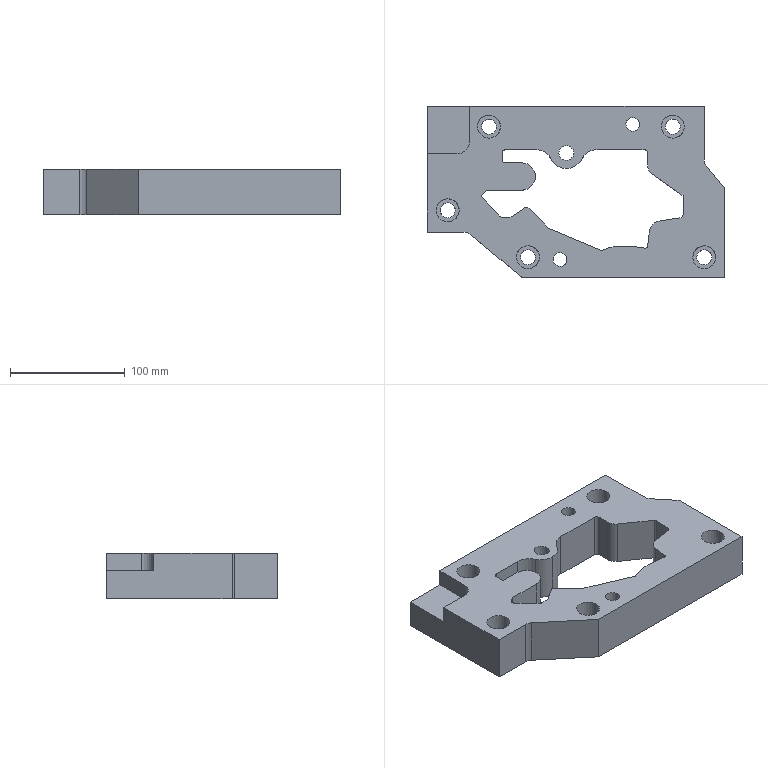Part | STEP file | gslz 2016.10.28-13_id490_x_t | 1 solid | 75 faces | box 260 x 150 x 40 mm | volume 956764 mm3 | cylinder 38 | plane 37 | commonest cylinder face diameters 4 x9 20 x7 13 x6 30 x4 6 x3 12 x3